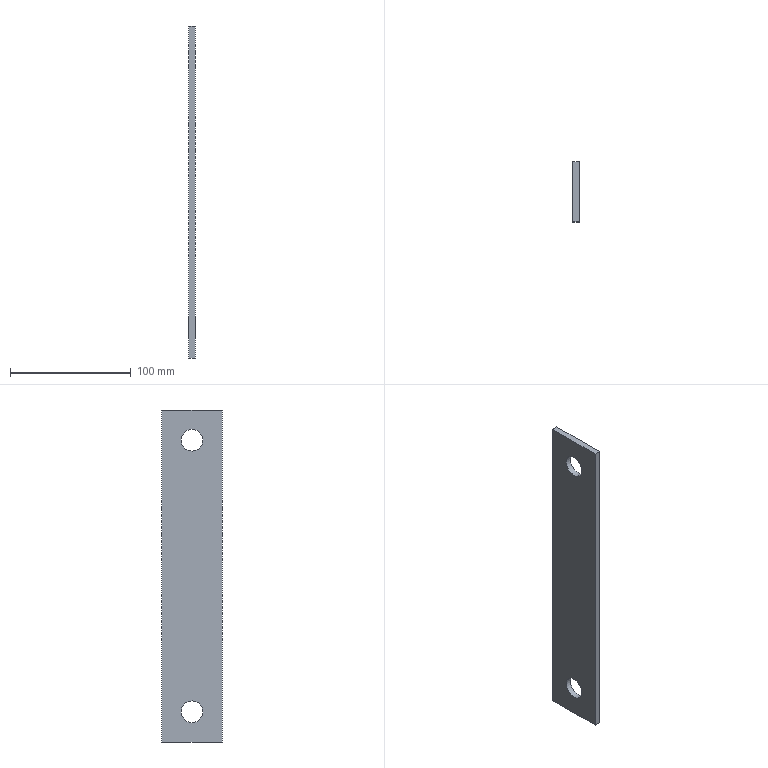Part | NX | features solid 2 | 1 solid | 8 faces | box 5 x 50 x 275 mm | volume 66205 mm3 | plane 6 | cylinder 2 | commonest cylinder face diameters 18 x2
STEP:
#1=CARTESIAN_POINT('',(1210.,610.,65.));
#2=VERTEX_POINT('',#1);
#3=CARTESIAN_POINT('',(1215.,610.,65.));
#4=VERTEX_POINT('',#3);
#5=CARTESIAN_POINT('',(1200.,610.,65.));
#6=DIRECTION('',(1.,0.,0.));
#7=VECTOR('',#6,1000.);
#8=LINE('',#5,#7);
#9=EDGE_CURVE('',#2,#4,#8,.T.);
#10=ORIENTED_EDGE('',*,*,#9,.F.);
#11=CARTESIAN_POINT('',(1210.,560.,65.));
#12=VERTEX_POINT('',#11);
#13=CARTESIAN_POINT('',(1210.,560.,65.));
#14=DIRECTION('',(0.,-1.,0.));
#15=VECTOR('',#14,1000.);
#16=LINE('',#13,#15);
#17=EDGE_CURVE('',#12,#2,#16,.F.);
#18=ORIENTED_EDGE('',*,*,#17,.F.);
#19=CARTESIAN_POINT('',(1215.,560.,65.));
#20=VERTEX_POINT('',#19);
#21=CARTESIAN_POINT('',(1210.,560.,65.));
#22=DIRECTION('',(-1.,0.,0.));
#23=VECTOR('',#22,1000.);
#24=LINE('',#21,#23);
#25=EDGE_CURVE('',#12,#20,#24,.F.);
#26=ORIENTED_EDGE('',*,*,#25,.T.);
#27=CARTESIAN_POINT('',(1215.,560.,65.));
#28=DIRECTION('',(0.,-1.,0.));
#29=VECTOR('',#28,1000.);
#30=LINE('',#27,#29);
#31=EDGE_CURVE('',#20,#4,#30,.F.);
#32=ORIENTED_EDGE('',*,*,#31,.T.);
#33=EDGE_LOOP('',(#10,#18,#26,#32));
#34=FACE_BOUND('',#33,.T.);
#35=CARTESIAN_POINT('',(1200.,560.,65.));
#36=DIRECTION('',(0.,0.,1.));
#37=DIRECTION('',(0.,1.,0.));
#38=AXIS2_PLACEMENT_3D('',#35,#36,#37);
#39=PLANE('',#38);
#40=ADVANCED_FACE('',(#34),#39,.T.);
#41=ORIENTED_EDGE('',*,*,#25,.F.);
#42=CARTESIAN_POINT('',(1210.,560.,-210.));
#43=VERTEX_POINT('',#42);
#44=CARTESIAN_POINT('',(1210.,560.,-10.));
#45=DIRECTION('',(0.,0.,-1.));
#46=VECTOR('',#45,1000.);
#47=LINE('',#44,#46);
#48=EDGE_CURVE('',#12,#43,#47,.T.);
#49=ORIENTED_EDGE('',*,*,#48,.T.);
#50=CARTESIAN_POINT('',(1215.,560.,-210.));
#51=VERTEX_POINT('',#50);
#52=CARTESIAN_POINT('',(1210.,560.,-210.));
#53=DIRECTION('',(-1.,0.,0.));
#54=VECTOR('',#53,1000.);
#55=LINE('',#52,#54);
#56=EDGE_CURVE('',#43,#51,#55,.F.);
#57=ORIENTED_EDGE('',*,*,#56,.T.);
#58=CARTESIAN_POINT('',(1215.,560.,-10.));
#59=DIRECTION('',(0.,0.,1.));
#60=VECTOR('',#59,1000.);
#61=LINE('',#58,#60);
#62=EDGE_CURVE('',#20,#51,#61,.F.);
#63=ORIENTED_EDGE('',*,*,#62,.F.);
#64=EDGE_LOOP('',(#41,#49,#57,#63));
#65=FACE_BOUND('',#64,.T.);
#66=CARTESIAN_POINT('',(1210.,560.,-10.));
#67=DIRECTION('',(0.,1.,0.));
#68=DIRECTION('',(0.,0.,-1.));
#69=AXIS2_PLACEMENT_3D('',#66,#67,#68);
#70=PLANE('',#69);
#71=ADVANCED_FACE('',(#65),#70,.F.);
#72=ORIENTED_EDGE('',*,*,#56,.F.);
#73=CARTESIAN_POINT('',(1210.,610.,-210.));
#74=VERTEX_POINT('',#73);
#75=CARTESIAN_POINT('',(1210.,560.,-210.));
#76=DIRECTION('',(0.,1.,0.));
#77=VECTOR('',#76,1000.);
#78=LINE('',#75,#77);
#79=EDGE_CURVE('',#43,#74,#78,.T.);
#80=ORIENTED_EDGE('',*,*,#79,.T.);
#81=CARTESIAN_POINT('',(1215.,610.,-210.));
#82=VERTEX_POINT('',#81);
#83=CARTESIAN_POINT('',(1210.,610.,-210.));
#84=DIRECTION('',(-1.,0.,0.));
#85=VECTOR('',#84,1000.);
#86=LINE('',#83,#85);
#87=EDGE_CURVE('',#74,#82,#86,.F.);
#88=ORIENTED_EDGE('',*,*,#87,.T.);
#89=CARTESIAN_POINT('',(1215.,560.,-210.));
#90=DIRECTION('',(0.,1.,0.));
#91=VECTOR('',#90,1000.);
#92=LINE('',#89,#91);
#93=EDGE_CURVE('',#51,#82,#92,.T.);
#94=ORIENTED_EDGE('',*,*,#93,.F.);
#95=EDGE_LOOP('',(#72,#80,#88,#94));
#96=FACE_BOUND('',#95,.T.);
#97=CARTESIAN_POINT('',(1210.,560.,-210.));
#98=DIRECTION('',(0.,0.,1.));
#99=DIRECTION('',(0.,1.,0.));
#100=AXIS2_PLACEMENT_3D('',#97,#98,#99);
#101=PLANE('',#100);
#102=ADVANCED_FACE('',(#96),#101,.F.);
#103=CARTESIAN_POINT('',(1210.,610.,-10.));
#104=DIRECTION('',(0.,0.,-1.));
#105=VECTOR('',#104,1000.);
#106=LINE('',#103,#105);
#107=EDGE_CURVE('',#2,#74,#106,.T.);
#108=ORIENTED_EDGE('',*,*,#107,.F.);
#109=ORIENTED_EDGE('',*,*,#9,.T.);
#110=CARTESIAN_POINT('',(1215.,610.,-10.));
#111=DIRECTION('',(0.,0.,1.));
#112=VECTOR('',#111,1000.);
#113=LINE('',#110,#112);
#114=EDGE_CURVE('',#4,#82,#113,.F.);
#115=ORIENTED_EDGE('',*,*,#114,.T.);
#116=ORIENTED_EDGE('',*,*,#87,.F.);
#117=EDGE_LOOP('',(#108,#109,#115,#116));
#118=FACE_BOUND('',#117,.T.);
#119=CARTESIAN_POINT('',(1210.,610.,-10.));
#120=DIRECTION('',(0.,1.,0.));
#121=DIRECTION('',(0.,0.,-1.));
#122=AXIS2_PLACEMENT_3D('',#119,#120,#121);
#123=PLANE('',#122);
#124=ADVANCED_FACE('',(#118),#123,.T.);
#125=CARTESIAN_POINT('',(1215.,585.,49.));
#126=VERTEX_POINT('',#125);
#127=CARTESIAN_POINT('',(1215.,585.,40.));
#128=DIRECTION('',(1.,0.,0.));
#129=DIRECTION('',(0.,0.,1.));
#130=AXIS2_PLACEMENT_3D('',#127,#128,#129);
#131=CIRCLE('',#130,9.);
#132=EDGE_CURVE('',#126,#126,#131,.T.);
#133=ORIENTED_EDGE('',*,*,#132,.F.);
#134=EDGE_LOOP('',(#133));
#135=FACE_BOUND('',#134,.T.);
#136=CARTESIAN_POINT('',(1215.,585.,-176.));
#137=VERTEX_POINT('',#136);
#138=CARTESIAN_POINT('',(1215.,585.,-185.));
#139=DIRECTION('',(1.,0.,0.));
#140=DIRECTION('',(0.,0.,1.));
#141=AXIS2_PLACEMENT_3D('',#138,#139,#140);
#142=CIRCLE('',#141,9.);
#143=EDGE_CURVE('',#137,#137,#142,.T.);
#144=ORIENTED_EDGE('',*,*,#143,.F.);
#145=EDGE_LOOP('',(#144));
#146=FACE_BOUND('',#145,.T.);
#147=ORIENTED_EDGE('',*,*,#93,.T.);
#148=ORIENTED_EDGE('',*,*,#114,.F.);
#149=ORIENTED_EDGE('',*,*,#31,.F.);
#150=ORIENTED_EDGE('',*,*,#62,.T.);
#151=EDGE_LOOP('',(#147,#148,#149,#150));
#152=FACE_BOUND('',#151,.T.);
#153=CARTESIAN_POINT('',(1215.,560.,-10.));
#154=DIRECTION('',(1.,0.,0.));
#155=DIRECTION('',(0.,0.,1.));
#156=AXIS2_PLACEMENT_3D('',#153,#154,#155);
#157=PLANE('',#156);
#158=ADVANCED_FACE('',(#135,#146,#152),#157,.T.);
#159=CARTESIAN_POINT('',(1210.,585.,31.));
#160=VERTEX_POINT('',#159);
#161=CARTESIAN_POINT('',(1210.,585.,40.));
#162=DIRECTION('',(-1.,0.,0.));
#163=DIRECTION('',(0.,0.,-1.));
#164=AXIS2_PLACEMENT_3D('',#161,#162,#163);
#165=CIRCLE('',#164,9.);
#166=EDGE_CURVE('',#160,#160,#165,.T.);
#167=ORIENTED_EDGE('',*,*,#166,.F.);
#168=EDGE_LOOP('',(#167));
#169=FACE_BOUND('',#168,.T.);
#170=CARTESIAN_POINT('',(1210.,585.,-194.));
#171=VERTEX_POINT('',#170);
#172=CARTESIAN_POINT('',(1210.,585.,-185.));
#173=DIRECTION('',(-1.,0.,0.));
#174=DIRECTION('',(0.,0.,-1.));
#175=AXIS2_PLACEMENT_3D('',#172,#173,#174);
#176=CIRCLE('',#175,9.);
#177=EDGE_CURVE('',#171,#171,#176,.T.);
#178=ORIENTED_EDGE('',*,*,#177,.F.);
#179=EDGE_LOOP('',(#178));
#180=FACE_BOUND('',#179,.T.);
#181=ORIENTED_EDGE('',*,*,#79,.F.);
#182=ORIENTED_EDGE('',*,*,#48,.F.);
#183=ORIENTED_EDGE('',*,*,#17,.T.);
#184=ORIENTED_EDGE('',*,*,#107,.T.);
#185=EDGE_LOOP('',(#181,#182,#183,#184));
#186=FACE_BOUND('',#185,.T.);
#187=CARTESIAN_POINT('',(1210.,560.,-10.));
#188=DIRECTION('',(1.,0.,0.));
#189=DIRECTION('',(0.,0.,1.));
#190=AXIS2_PLACEMENT_3D('',#187,#188,#189);
#191=PLANE('',#190);
#192=ADVANCED_FACE('',(#169,#180,#186),#191,.F.);
#193=ORIENTED_EDGE('',*,*,#143,.T.);
#194=EDGE_LOOP('',(#193));
#195=FACE_BOUND('',#194,.T.);
#196=ORIENTED_EDGE('',*,*,#177,.T.);
#197=EDGE_LOOP('',(#196));
#198=FACE_BOUND('',#197,.T.);
#199=CARTESIAN_POINT('',(1215.,585.,-185.));
#200=DIRECTION('',(-1.,0.,0.));
#201=DIRECTION('',(0.,0.,1.));
#202=AXIS2_PLACEMENT_3D('',#199,#200,#201);
#203=CYLINDRICAL_SURFACE('',#202,9.);
#204=ADVANCED_FACE('',(#195,#198),#203,.F.);
#205=ORIENTED_EDGE('',*,*,#132,.T.);
#206=EDGE_LOOP('',(#205));
#207=FACE_BOUND('',#206,.T.);
#208=ORIENTED_EDGE('',*,*,#166,.T.);
#209=EDGE_LOOP('',(#208));
#210=FACE_BOUND('',#209,.T.);
#211=CARTESIAN_POINT('',(1215.,585.,40.));
#212=DIRECTION('',(-1.,0.,0.));
#213=DIRECTION('',(0.,0.,1.));
#214=AXIS2_PLACEMENT_3D('',#211,#212,#213);
#215=CYLINDRICAL_SURFACE('',#214,9.);
#216=ADVANCED_FACE('',(#207,#210),#215,.F.);
#217=CLOSED_SHELL('',(#40,#71,#102,#124,#158,#192,#204,#216));
#218=MANIFOLD_SOLID_BREP('',#217);
#219=(LENGTH_UNIT()NAMED_UNIT(*)SI_UNIT(.MILLI.,.METRE.));
#220=UNCERTAINTY_MEASURE_WITH_UNIT(LENGTH_MEASURE(0.00001),#219,'','');
#221=(NAMED_UNIT(*)PLANE_ANGLE_UNIT()SI_UNIT($,.RADIAN.));
#222=(NAMED_UNIT(*)SI_UNIT($,.STERADIAN.)SOLID_ANGLE_UNIT());
#223=(GEOMETRIC_REPRESENTATION_CONTEXT(3)GLOBAL_UNCERTAINTY_ASSIGNED_CONTEXT((#220))GLOBAL_UNIT_ASSIGNED_CONTEXT((#219,#221,#222))REPRESENTATION_CONTEXT('',''));
#224=ADVANCED_BREP_SHAPE_REPRESENTATION('',(#218),#223);